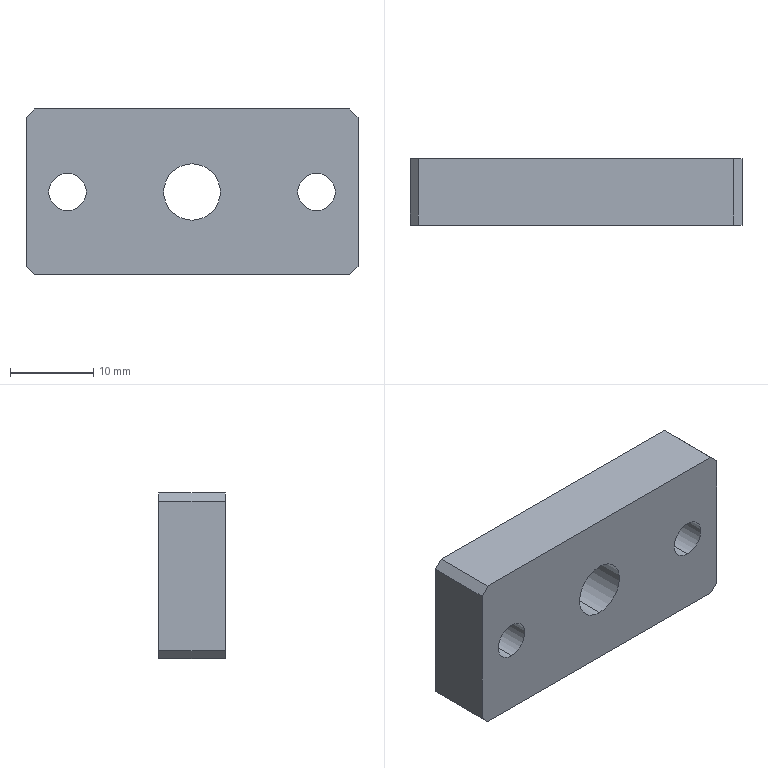Part | NX | features BREP 1 | 1 solid | 22 faces | box 40 x 8 x 20 mm | volume 5530 mm3 | plane 12 | cylinder 10 | commonest cylinder face diameters 4.5 x4 8 x4 6.8 x2
STEP:
#1=CARTESIAN_POINT('',(15.,-4.,-2.25));
#2=VERTEX_POINT('',#1);
#3=CARTESIAN_POINT('',(15.,-4.,2.25));
#4=VERTEX_POINT('',#3);
#5=CARTESIAN_POINT('',(15.,-4.,0.));
#6=DIRECTION('',(0.,1.,0.));
#7=DIRECTION('',(0.,0.,1.));
#8=AXIS2_PLACEMENT_3D('',#5,#6,#7);
#9=CIRCLE('',#8,2.25);
#10=EDGE_CURVE('',#2,#4,#9,.T.);
#11=ORIENTED_EDGE('',*,*,#10,.F.);
#12=CARTESIAN_POINT('',(15.,-0.5,-2.25));
#13=VERTEX_POINT('',#12);
#14=CARTESIAN_POINT('',(15.,4.,-2.25));
#15=DIRECTION('',(0.,1.,0.));
#16=VECTOR('',#15,1000.);
#17=LINE('',#14,#16);
#18=EDGE_CURVE('',#13,#2,#17,.F.);
#19=ORIENTED_EDGE('',*,*,#18,.F.);
#20=CARTESIAN_POINT('',(15.,-0.5,2.25));
#21=VERTEX_POINT('',#20);
#22=CARTESIAN_POINT('',(15.,-0.5,0.));
#23=DIRECTION('',(0.,1.,0.));
#24=DIRECTION('',(0.,0.,1.));
#25=AXIS2_PLACEMENT_3D('',#22,#23,#24);
#26=CIRCLE('',#25,2.25);
#27=EDGE_CURVE('',#13,#21,#26,.T.);
#28=ORIENTED_EDGE('',*,*,#27,.T.);
#29=CARTESIAN_POINT('',(15.,4.,2.25));
#30=DIRECTION('',(0.,1.,0.));
#31=VECTOR('',#30,1000.);
#32=LINE('',#29,#31);
#33=EDGE_CURVE('',#21,#4,#32,.F.);
#34=ORIENTED_EDGE('',*,*,#33,.T.);
#35=EDGE_LOOP('',(#11,#19,#28,#34));
#36=FACE_BOUND('',#35,.T.);
#37=CARTESIAN_POINT('',(15.,4.,0.));
#38=DIRECTION('',(0.,1.,0.));
#39=DIRECTION('',(0.,0.,1.));
#40=AXIS2_PLACEMENT_3D('',#37,#38,#39);
#41=CYLINDRICAL_SURFACE('',#40,2.25);
#42=ADVANCED_FACE('',(#36),#41,.F.);
#43=CARTESIAN_POINT('',(15.,-0.5,-4.));
#44=VERTEX_POINT('',#43);
#45=CARTESIAN_POINT('',(15.,-0.5,4.));
#46=VERTEX_POINT('',#45);
#47=CARTESIAN_POINT('',(15.,-0.5,0.));
#48=DIRECTION('',(0.,1.,0.));
#49=DIRECTION('',(0.,0.,1.));
#50=AXIS2_PLACEMENT_3D('',#47,#48,#49);
#51=CIRCLE('',#50,4.);
#52=EDGE_CURVE('',#44,#46,#51,.T.);
#53=ORIENTED_EDGE('',*,*,#52,.F.);
#54=CARTESIAN_POINT('',(15.,4.,-4.));
#55=VERTEX_POINT('',#54);
#56=CARTESIAN_POINT('',(15.,4.,-4.));
#57=DIRECTION('',(0.,1.,0.));
#58=VECTOR('',#57,1000.);
#59=LINE('',#56,#58);
#60=EDGE_CURVE('',#55,#44,#59,.F.);
#61=ORIENTED_EDGE('',*,*,#60,.F.);
#62=CARTESIAN_POINT('',(15.,4.,4.));
#63=VERTEX_POINT('',#62);
#64=CARTESIAN_POINT('',(15.,4.,0.));
#65=DIRECTION('',(0.,1.,0.));
#66=DIRECTION('',(0.,0.,1.));
#67=AXIS2_PLACEMENT_3D('',#64,#65,#66);
#68=CIRCLE('',#67,4.);
#69=EDGE_CURVE('',#55,#63,#68,.T.);
#70=ORIENTED_EDGE('',*,*,#69,.T.);
#71=CARTESIAN_POINT('',(15.,4.,4.));
#72=DIRECTION('',(0.,1.,0.));
#73=VECTOR('',#72,1000.);
#74=LINE('',#71,#73);
#75=EDGE_CURVE('',#63,#46,#74,.F.);
#76=ORIENTED_EDGE('',*,*,#75,.T.);
#77=EDGE_LOOP('',(#53,#61,#70,#76));
#78=FACE_BOUND('',#77,.T.);
#79=CARTESIAN_POINT('',(15.,4.,0.));
#80=DIRECTION('',(0.,1.,0.));
#81=DIRECTION('',(0.,0.,1.));
#82=AXIS2_PLACEMENT_3D('',#79,#80,#81);
#83=CYLINDRICAL_SURFACE('',#82,4.);
#84=ADVANCED_FACE('',(#78),#83,.F.);
#85=CARTESIAN_POINT('',(-15.,-4.,-2.25));
#86=VERTEX_POINT('',#85);
#87=CARTESIAN_POINT('',(-15.,-4.,2.25));
#88=VERTEX_POINT('',#87);
#89=CARTESIAN_POINT('',(-15.,-4.,0.));
#90=DIRECTION('',(0.,1.,0.));
#91=DIRECTION('',(0.,0.,1.));
#92=AXIS2_PLACEMENT_3D('',#89,#90,#91);
#93=CIRCLE('',#92,2.25);
#94=EDGE_CURVE('',#86,#88,#93,.T.);
#95=ORIENTED_EDGE('',*,*,#94,.F.);
#96=CARTESIAN_POINT('',(-15.,-0.5,-2.25));
#97=VERTEX_POINT('',#96);
#98=CARTESIAN_POINT('',(-15.,4.,-2.25));
#99=DIRECTION('',(0.,1.,0.));
#100=VECTOR('',#99,1000.);
#101=LINE('',#98,#100);
#102=EDGE_CURVE('',#97,#86,#101,.F.);
#103=ORIENTED_EDGE('',*,*,#102,.F.);
#104=CARTESIAN_POINT('',(-15.,-0.5,2.25));
#105=VERTEX_POINT('',#104);
#106=CARTESIAN_POINT('',(-15.,-0.5,0.));
#107=DIRECTION('',(0.,1.,0.));
#108=DIRECTION('',(0.,0.,1.));
#109=AXIS2_PLACEMENT_3D('',#106,#107,#108);
#110=CIRCLE('',#109,2.25);
#111=EDGE_CURVE('',#97,#105,#110,.T.);
#112=ORIENTED_EDGE('',*,*,#111,.T.);
#113=CARTESIAN_POINT('',(-15.,4.,2.25));
#114=DIRECTION('',(0.,1.,0.));
#115=VECTOR('',#114,1000.);
#116=LINE('',#113,#115);
#117=EDGE_CURVE('',#105,#88,#116,.F.);
#118=ORIENTED_EDGE('',*,*,#117,.T.);
#119=EDGE_LOOP('',(#95,#103,#112,#118));
#120=FACE_BOUND('',#119,.T.);
#121=CARTESIAN_POINT('',(-15.,4.,0.));
#122=DIRECTION('',(0.,1.,0.));
#123=DIRECTION('',(0.,0.,1.));
#124=AXIS2_PLACEMENT_3D('',#121,#122,#123);
#125=CYLINDRICAL_SURFACE('',#124,2.25);
#126=ADVANCED_FACE('',(#120),#125,.F.);
#127=CARTESIAN_POINT('',(-15.,-0.5,-4.));
#128=VERTEX_POINT('',#127);
#129=CARTESIAN_POINT('',(-15.,-0.5,4.));
#130=VERTEX_POINT('',#129);
#131=CARTESIAN_POINT('',(-15.,-0.5,0.));
#132=DIRECTION('',(0.,1.,0.));
#133=DIRECTION('',(0.,0.,1.));
#134=AXIS2_PLACEMENT_3D('',#131,#132,#133);
#135=CIRCLE('',#134,4.);
#136=EDGE_CURVE('',#128,#130,#135,.T.);
#137=ORIENTED_EDGE('',*,*,#136,.F.);
#138=CARTESIAN_POINT('',(-15.,4.,-4.));
#139=VERTEX_POINT('',#138);
#140=CARTESIAN_POINT('',(-15.,4.,-4.));
#141=DIRECTION('',(0.,1.,0.));
#142=VECTOR('',#141,1000.);
#143=LINE('',#140,#142);
#144=EDGE_CURVE('',#139,#128,#143,.F.);
#145=ORIENTED_EDGE('',*,*,#144,.F.);
#146=CARTESIAN_POINT('',(-15.,4.,4.));
#147=VERTEX_POINT('',#146);
#148=CARTESIAN_POINT('',(-15.,4.,0.));
#149=DIRECTION('',(0.,1.,0.));
#150=DIRECTION('',(0.,0.,1.));
#151=AXIS2_PLACEMENT_3D('',#148,#149,#150);
#152=CIRCLE('',#151,4.);
#153=EDGE_CURVE('',#139,#147,#152,.T.);
#154=ORIENTED_EDGE('',*,*,#153,.T.);
#155=CARTESIAN_POINT('',(-15.,4.,4.));
#156=DIRECTION('',(0.,1.,0.));
#157=VECTOR('',#156,1000.);
#158=LINE('',#155,#157);
#159=EDGE_CURVE('',#147,#130,#158,.F.);
#160=ORIENTED_EDGE('',*,*,#159,.T.);
#161=EDGE_LOOP('',(#137,#145,#154,#160));
#162=FACE_BOUND('',#161,.T.);
#163=CARTESIAN_POINT('',(-15.,4.,0.));
#164=DIRECTION('',(0.,1.,0.));
#165=DIRECTION('',(0.,0.,1.));
#166=AXIS2_PLACEMENT_3D('',#163,#164,#165);
#167=CYLINDRICAL_SURFACE('',#166,4.);
#168=ADVANCED_FACE('',(#162),#167,.F.);
#169=CARTESIAN_POINT('',(0.,-4.,-3.4));
#170=VERTEX_POINT('',#169);
#171=CARTESIAN_POINT('',(0.,-4.,3.4));
#172=VERTEX_POINT('',#171);
#173=CARTESIAN_POINT('',(0.,-4.,0.));
#174=DIRECTION('',(0.,1.,0.));
#175=DIRECTION('',(0.,0.,1.));
#176=AXIS2_PLACEMENT_3D('',#173,#174,#175);
#177=CIRCLE('',#176,3.4);
#178=EDGE_CURVE('',#170,#172,#177,.T.);
#179=ORIENTED_EDGE('',*,*,#178,.F.);
#180=CARTESIAN_POINT('',(0.,4.,-3.4));
#181=VERTEX_POINT('',#180);
#182=CARTESIAN_POINT('',(0.,4.,-3.4));
#183=DIRECTION('',(0.,1.,0.));
#184=VECTOR('',#183,1000.);
#185=LINE('',#182,#184);
#186=EDGE_CURVE('',#181,#170,#185,.F.);
#187=ORIENTED_EDGE('',*,*,#186,.F.);
#188=CARTESIAN_POINT('',(0.,4.,3.4));
#189=VERTEX_POINT('',#188);
#190=CARTESIAN_POINT('',(0.,4.,0.));
#191=DIRECTION('',(0.,1.,0.));
#192=DIRECTION('',(0.,0.,1.));
#193=AXIS2_PLACEMENT_3D('',#190,#191,#192);
#194=CIRCLE('',#193,3.4);
#195=EDGE_CURVE('',#181,#189,#194,.T.);
#196=ORIENTED_EDGE('',*,*,#195,.T.);
#197=CARTESIAN_POINT('',(0.,4.,3.4));
#198=DIRECTION('',(0.,1.,0.));
#199=VECTOR('',#198,1000.);
#200=LINE('',#197,#199);
#201=EDGE_CURVE('',#189,#172,#200,.F.);
#202=ORIENTED_EDGE('',*,*,#201,.T.);
#203=EDGE_LOOP('',(#179,#187,#196,#202));
#204=FACE_BOUND('',#203,.T.);
#205=CARTESIAN_POINT('',(0.,4.,0.));
#206=DIRECTION('',(0.,1.,0.));
#207=DIRECTION('',(0.,0.,1.));
#208=AXIS2_PLACEMENT_3D('',#205,#206,#207);
#209=CYLINDRICAL_SURFACE('',#208,3.4);
#210=ADVANCED_FACE('',(#204),#209,.F.);
#211=CARTESIAN_POINT('',(19.,-4.,-10.));
#212=VERTEX_POINT('',#211);
#213=CARTESIAN_POINT('',(-19.,-4.,-10.));
#214=VERTEX_POINT('',#213);
#215=CARTESIAN_POINT('',(20.,-4.,-10.));
#216=DIRECTION('',(-1.,0.,0.));
#217=VECTOR('',#216,1000.);
#218=LINE('',#215,#217);
#219=EDGE_CURVE('',#212,#214,#218,.T.);
#220=ORIENTED_EDGE('',*,*,#219,.F.);
#221=CARTESIAN_POINT('',(20.,-4.,-9.));
#222=VERTEX_POINT('',#221);
#223=CARTESIAN_POINT('',(29.5,-4.,0.5));
#224=DIRECTION('',(0.7071,0.,0.7071));
#225=VECTOR('',#224,1000.);
#226=LINE('',#223,#225);
#227=EDGE_CURVE('',#212,#222,#226,.T.);
#228=ORIENTED_EDGE('',*,*,#227,.T.);
#229=CARTESIAN_POINT('',(20.,-4.,9.));
#230=VERTEX_POINT('',#229);
#231=CARTESIAN_POINT('',(20.,-4.,-10.));
#232=DIRECTION('',(0.,0.,-1.));
#233=VECTOR('',#232,1000.);
#234=LINE('',#231,#233);
#235=EDGE_CURVE('',#230,#222,#234,.T.);
#236=ORIENTED_EDGE('',*,*,#235,.F.);
#237=CARTESIAN_POINT('',(19.,-4.,10.));
#238=VERTEX_POINT('',#237);
#239=CARTESIAN_POINT('',(19.5,-4.,9.5));
#240=DIRECTION('',(-0.7071,0.,0.7071));
#241=VECTOR('',#240,1000.);
#242=LINE('',#239,#241);
#243=EDGE_CURVE('',#230,#238,#242,.T.);
#244=ORIENTED_EDGE('',*,*,#243,.T.);
#245=CARTESIAN_POINT('',(-19.,-4.,10.));
#246=VERTEX_POINT('',#245);
#247=CARTESIAN_POINT('',(20.,-4.,10.));
#248=DIRECTION('',(1.,0.,0.));
#249=VECTOR('',#248,1000.);
#250=LINE('',#247,#249);
#251=EDGE_CURVE('',#246,#238,#250,.T.);
#252=ORIENTED_EDGE('',*,*,#251,.F.);
#253=CARTESIAN_POINT('',(-20.,-4.,9.));
#254=VERTEX_POINT('',#253);
#255=CARTESIAN_POINT('',(0.5,-4.,29.5));
#256=DIRECTION('',(-0.7071,0.,-0.7071));
#257=VECTOR('',#256,1000.);
#258=LINE('',#255,#257);
#259=EDGE_CURVE('',#246,#254,#258,.T.);
#260=ORIENTED_EDGE('',*,*,#259,.T.);
#261=CARTESIAN_POINT('',(-20.,-4.,-9.));
#262=VERTEX_POINT('',#261);
#263=CARTESIAN_POINT('',(-20.,-4.,-10.));
#264=DIRECTION('',(0.,0.,1.));
#265=VECTOR('',#264,1000.);
#266=LINE('',#263,#265);
#267=EDGE_CURVE('',#262,#254,#266,.T.);
#268=ORIENTED_EDGE('',*,*,#267,.F.);
#269=CARTESIAN_POINT('',(-9.5,-4.,-19.5));
#270=DIRECTION('',(0.7071,0.,-0.7071));
#271=VECTOR('',#270,1000.);
#272=LINE('',#269,#271);
#273=EDGE_CURVE('',#262,#214,#272,.T.);
#274=ORIENTED_EDGE('',*,*,#273,.T.);
#275=EDGE_LOOP('',(#220,#228,#236,#244,#252,#260,#268,#274));
#276=FACE_BOUND('',#275,.T.);
#277=CARTESIAN_POINT('',(-15.,-4.,0.));
#278=DIRECTION('',(0.,1.,0.));
#279=DIRECTION('',(0.,0.,1.));
#280=AXIS2_PLACEMENT_3D('',#277,#278,#279);
#281=CIRCLE('',#280,2.25);
#282=EDGE_CURVE('',#88,#86,#281,.T.);
#283=ORIENTED_EDGE('',*,*,#282,.T.);
#284=ORIENTED_EDGE('',*,*,#94,.T.);
#285=EDGE_LOOP('',(#283,#284));
#286=FACE_BOUND('',#285,.T.);
#287=CARTESIAN_POINT('',(0.,-4.,0.));
#288=DIRECTION('',(0.,1.,0.));
#289=DIRECTION('',(0.,0.,1.));
#290=AXIS2_PLACEMENT_3D('',#287,#288,#289);
#291=CIRCLE('',#290,3.4);
#292=EDGE_CURVE('',#172,#170,#291,.T.);
#293=ORIENTED_EDGE('',*,*,#292,.T.);
#294=ORIENTED_EDGE('',*,*,#178,.T.);
#295=EDGE_LOOP('',(#293,#294));
#296=FACE_BOUND('',#295,.T.);
#297=CARTESIAN_POINT('',(15.,-4.,0.));
#298=DIRECTION('',(0.,1.,0.));
#299=DIRECTION('',(0.,0.,1.));
#300=AXIS2_PLACEMENT_3D('',#297,#298,#299);
#301=CIRCLE('',#300,2.25);
#302=EDGE_CURVE('',#4,#2,#301,.T.);
#303=ORIENTED_EDGE('',*,*,#302,.T.);
#304=ORIENTED_EDGE('',*,*,#10,.T.);
#305=EDGE_LOOP('',(#303,#304));
#306=FACE_BOUND('',#305,.T.);
#307=CARTESIAN_POINT('',(20.,-4.,10.));
#308=DIRECTION('',(0.,-1.,0.));
#309=DIRECTION('',(0.,0.,-1.));
#310=AXIS2_PLACEMENT_3D('',#307,#308,#309);
#311=PLANE('',#310);
#312=ADVANCED_FACE('',(#276,#286,#296,#306),#311,.T.);
#313=ORIENTED_EDGE('',*,*,#235,.T.);
#314=CARTESIAN_POINT('',(20.,4.,-9.));
#315=VERTEX_POINT('',#314);
#316=CARTESIAN_POINT('',(20.,4.,-9.));
#317=DIRECTION('',(0.,1.,0.));
#318=VECTOR('',#317,1000.);
#319=LINE('',#316,#318);
#320=EDGE_CURVE('',#222,#315,#319,.T.);
#321=ORIENTED_EDGE('',*,*,#320,.T.);
#322=CARTESIAN_POINT('',(20.,4.,9.));
#323=VERTEX_POINT('',#322);
#324=CARTESIAN_POINT('',(20.,4.,-10.));
#325=DIRECTION('',(0.,0.,-1.));
#326=VECTOR('',#325,1000.);
#327=LINE('',#324,#326);
#328=EDGE_CURVE('',#323,#315,#327,.T.);
#329=ORIENTED_EDGE('',*,*,#328,.F.);
#330=CARTESIAN_POINT('',(20.,4.,9.));
#331=DIRECTION('',(0.,-1.,0.));
#332=VECTOR('',#331,1000.);
#333=LINE('',#330,#332);
#334=EDGE_CURVE('',#323,#230,#333,.T.);
#335=ORIENTED_EDGE('',*,*,#334,.T.);
#336=EDGE_LOOP('',(#313,#321,#329,#335));
#337=FACE_BOUND('',#336,.T.);
#338=CARTESIAN_POINT('',(20.,4.,-10.));
#339=DIRECTION('',(-1.,0.,0.));
#340=DIRECTION('',(0.,0.,1.));
#341=AXIS2_PLACEMENT_3D('',#338,#339,#340);
#342=PLANE('',#341);
#343=ADVANCED_FACE('',(#337),#342,.F.);
#344=CARTESIAN_POINT('',(19.,4.,-10.));
#345=VERTEX_POINT('',#344);
#346=CARTESIAN_POINT('',(-19.,4.,-10.));
#347=VERTEX_POINT('',#346);
#348=CARTESIAN_POINT('',(20.,4.,-10.));
#349=DIRECTION('',(-1.,0.,0.));
#350=VECTOR('',#349,1000.);
#351=LINE('',#348,#350);
#352=EDGE_CURVE('',#345,#347,#351,.T.);
#353=ORIENTED_EDGE('',*,*,#352,.F.);
#354=CARTESIAN_POINT('',(19.,4.,-10.));
#355=DIRECTION('',(0.,-1.,0.));
#356=VECTOR('',#355,1000.);
#357=LINE('',#354,#356);
#358=EDGE_CURVE('',#345,#212,#357,.T.);
#359=ORIENTED_EDGE('',*,*,#358,.T.);
#360=ORIENTED_EDGE('',*,*,#219,.T.);
#361=CARTESIAN_POINT('',(-19.,4.,-10.));
#362=DIRECTION('',(0.,1.,0.));
#363=VECTOR('',#362,1000.);
#364=LINE('',#361,#363);
#365=EDGE_CURVE('',#214,#347,#364,.T.);
#366=ORIENTED_EDGE('',*,*,#365,.T.);
#367=EDGE_LOOP('',(#353,#359,#360,#366));
#368=FACE_BOUND('',#367,.T.);
#369=CARTESIAN_POINT('',(20.,4.,-10.));
#370=DIRECTION('',(0.,0.,1.));
#371=DIRECTION('',(1.,0.,0.));
#372=AXIS2_PLACEMENT_3D('',#369,#370,#371);
#373=PLANE('',#372);
#374=ADVANCED_FACE('',(#368),#373,.F.);
#375=CARTESIAN_POINT('',(-20.,4.,-9.));
#376=VERTEX_POINT('',#375);
#377=CARTESIAN_POINT('',(-20.,4.,9.));
#378=VERTEX_POINT('',#377);
#379=CARTESIAN_POINT('',(-20.,4.,-10.));
#380=DIRECTION('',(0.,0.,1.));
#381=VECTOR('',#380,1000.);
#382=LINE('',#379,#381);
#383=EDGE_CURVE('',#376,#378,#382,.T.);
#384=ORIENTED_EDGE('',*,*,#383,.F.);
#385=CARTESIAN_POINT('',(-20.,4.,-9.));
#386=DIRECTION('',(0.,-1.,0.));
#387=VECTOR('',#386,1000.);
#388=LINE('',#385,#387);
#389=EDGE_CURVE('',#376,#262,#388,.T.);
#390=ORIENTED_EDGE('',*,*,#389,.T.);
#391=ORIENTED_EDGE('',*,*,#267,.T.);
#392=CARTESIAN_POINT('',(-20.,4.,9.));
#393=DIRECTION('',(0.,1.,0.));
#394=VECTOR('',#393,1000.);
#395=LINE('',#392,#394);
#396=EDGE_CURVE('',#254,#378,#395,.T.);
#397=ORIENTED_EDGE('',*,*,#396,.T.);
#398=EDGE_LOOP('',(#384,#390,#391,#397));
#399=FACE_BOUND('',#398,.T.);
#400=CARTESIAN_POINT('',(-20.,4.,-10.));
#401=DIRECTION('',(1.,0.,0.));
#402=DIRECTION('',(0.,0.,1.));
#403=AXIS2_PLACEMENT_3D('',#400,#401,#402);
#404=PLANE('',#403);
#405=ADVANCED_FACE('',(#399),#404,.F.);
#406=ORIENTED_EDGE('',*,*,#251,.T.);
#407=CARTESIAN_POINT('',(19.,4.,10.));
#408=VERTEX_POINT('',#407);
#409=CARTESIAN_POINT('',(19.,4.,10.));
#410=DIRECTION('',(0.,1.,0.));
#411=VECTOR('',#410,1000.);
#412=LINE('',#409,#411);
#413=EDGE_CURVE('',#238,#408,#412,.T.);
#414=ORIENTED_EDGE('',*,*,#413,.T.);
#415=CARTESIAN_POINT('',(-19.,4.,10.));
#416=VERTEX_POINT('',#415);
#417=CARTESIAN_POINT('',(20.,4.,10.));
#418=DIRECTION('',(1.,0.,0.));
#419=VECTOR('',#418,1000.);
#420=LINE('',#417,#419);
#421=EDGE_CURVE('',#416,#408,#420,.T.);
#422=ORIENTED_EDGE('',*,*,#421,.F.);
#423=CARTESIAN_POINT('',(-19.,4.,10.));
#424=DIRECTION('',(0.,-1.,0.));
#425=VECTOR('',#424,1000.);
#426=LINE('',#423,#425);
#427=EDGE_CURVE('',#416,#246,#426,.T.);
#428=ORIENTED_EDGE('',*,*,#427,.T.);
#429=EDGE_LOOP('',(#406,#414,#422,#428));
#430=FACE_BOUND('',#429,.T.);
#431=CARTESIAN_POINT('',(20.,4.,10.));
#432=DIRECTION('',(0.,0.,-1.));
#433=DIRECTION('',(-1.,0.,0.));
#434=AXIS2_PLACEMENT_3D('',#431,#432,#433);
#435=PLANE('',#434);
#436=ADVANCED_FACE('',(#430),#435,.F.);
#437=ORIENTED_EDGE('',*,*,#328,.T.);
#438=CARTESIAN_POINT('',(19.,4.,-10.));
#439=DIRECTION('',(-0.7071,0.,-0.7071));
#440=VECTOR('',#439,1000.);
#441=LINE('',#438,#440);
#442=EDGE_CURVE('',#315,#345,#441,.T.);
#443=ORIENTED_EDGE('',*,*,#442,.T.);
#444=ORIENTED_EDGE('',*,*,#352,.T.);
#445=CARTESIAN_POINT('',(-20.,4.,-9.));
#446=DIRECTION('',(-0.7071,0.,0.7071));
#447=VECTOR('',#446,1000.);
#448=LINE('',#445,#447);
#449=EDGE_CURVE('',#347,#376,#448,.T.);
#450=ORIENTED_EDGE('',*,*,#449,.T.);
#451=ORIENTED_EDGE('',*,*,#383,.T.);
#452=CARTESIAN_POINT('',(-19.,4.,10.));
#453=DIRECTION('',(0.7071,0.,0.7071));
#454=VECTOR('',#453,1000.);
#455=LINE('',#452,#454);
#456=EDGE_CURVE('',#378,#416,#455,.T.);
#457=ORIENTED_EDGE('',*,*,#456,.T.);
#458=ORIENTED_EDGE('',*,*,#421,.T.);
#459=CARTESIAN_POINT('',(20.,4.,9.));
#460=DIRECTION('',(0.7071,0.,-0.7071));
#461=VECTOR('',#460,1000.);
#462=LINE('',#459,#461);
#463=EDGE_CURVE('',#408,#323,#462,.T.);
#464=ORIENTED_EDGE('',*,*,#463,.T.);
#465=EDGE_LOOP('',(#437,#443,#444,#450,#451,#457,#458,#464));
#466=FACE_BOUND('',#465,.T.);
#467=CARTESIAN_POINT('',(15.,4.,0.));
#468=DIRECTION('',(0.,1.,0.));
#469=DIRECTION('',(0.,0.,1.));
#470=AXIS2_PLACEMENT_3D('',#467,#468,#469);
#471=CIRCLE('',#470,4.);
#472=EDGE_CURVE('',#63,#55,#471,.T.);
#473=ORIENTED_EDGE('',*,*,#472,.F.);
#474=ORIENTED_EDGE('',*,*,#69,.F.);
#475=EDGE_LOOP('',(#473,#474));
#476=FACE_BOUND('',#475,.T.);
#477=CARTESIAN_POINT('',(-15.,4.,0.));
#478=DIRECTION('',(0.,1.,0.));
#479=DIRECTION('',(0.,0.,1.));
#480=AXIS2_PLACEMENT_3D('',#477,#478,#479);
#481=CIRCLE('',#480,4.);
#482=EDGE_CURVE('',#147,#139,#481,.T.);
#483=ORIENTED_EDGE('',*,*,#482,.F.);
#484=ORIENTED_EDGE('',*,*,#153,.F.);
#485=EDGE_LOOP('',(#483,#484));
#486=FACE_BOUND('',#485,.T.);
#487=CARTESIAN_POINT('',(0.,4.,0.));
#488=DIRECTION('',(0.,1.,0.));
#489=DIRECTION('',(0.,0.,1.));
#490=AXIS2_PLACEMENT_3D('',#487,#488,#489);
#491=CIRCLE('',#490,3.4);
#492=EDGE_CURVE('',#189,#181,#491,.T.);
#493=ORIENTED_EDGE('',*,*,#492,.F.);
#494=ORIENTED_EDGE('',*,*,#195,.F.);
#495=EDGE_LOOP('',(#493,#494));
#496=FACE_BOUND('',#495,.T.);
#497=CARTESIAN_POINT('',(20.,4.,10.));
#498=DIRECTION('',(0.,-1.,0.));
#499=DIRECTION('',(0.,0.,-1.));
#500=AXIS2_PLACEMENT_3D('',#497,#498,#499);
#501=PLANE('',#500);
#502=ADVANCED_FACE('',(#466,#476,#486,#496),#501,.F.);
#503=ORIENTED_EDGE('',*,*,#442,.F.);
#504=ORIENTED_EDGE('',*,*,#320,.F.);
#505=ORIENTED_EDGE('',*,*,#227,.F.);
#506=ORIENTED_EDGE('',*,*,#358,.F.);
#507=EDGE_LOOP('',(#503,#504,#505,#506));
#508=FACE_BOUND('',#507,.T.);
#509=CARTESIAN_POINT('',(19.,4.,-10.));
#510=DIRECTION('',(-0.7071,0.,0.7071));
#511=DIRECTION('',(0.,1.,0.));
#512=AXIS2_PLACEMENT_3D('',#509,#510,#511);
#513=PLANE('',#512);
#514=ADVANCED_FACE('',(#508),#513,.F.);
#515=ORIENTED_EDGE('',*,*,#463,.F.);
#516=ORIENTED_EDGE('',*,*,#413,.F.);
#517=ORIENTED_EDGE('',*,*,#243,.F.);
#518=ORIENTED_EDGE('',*,*,#334,.F.);
#519=EDGE_LOOP('',(#515,#516,#517,#518));
#520=FACE_BOUND('',#519,.T.);
#521=CARTESIAN_POINT('',(20.,4.,9.));
#522=DIRECTION('',(-0.7071,0.,-0.7071));
#523=DIRECTION('',(-0.7071,0.,0.7071));
#524=AXIS2_PLACEMENT_3D('',#521,#522,#523);
#525=PLANE('',#524);
#526=ADVANCED_FACE('',(#520),#525,.F.);
#527=ORIENTED_EDGE('',*,*,#449,.F.);
#528=ORIENTED_EDGE('',*,*,#365,.F.);
#529=ORIENTED_EDGE('',*,*,#273,.F.);
#530=ORIENTED_EDGE('',*,*,#389,.F.);
#531=EDGE_LOOP('',(#527,#528,#529,#530));
#532=FACE_BOUND('',#531,.T.);
#533=CARTESIAN_POINT('',(-20.,4.,-9.));
#534=DIRECTION('',(0.7071,0.,0.7071));
#535=DIRECTION('',(0.,-1.,0.));
#536=AXIS2_PLACEMENT_3D('',#533,#534,#535);
#537=PLANE('',#536);
#538=ADVANCED_FACE('',(#532),#537,.F.);
#539=ORIENTED_EDGE('',*,*,#456,.F.);
#540=ORIENTED_EDGE('',*,*,#396,.F.);
#541=ORIENTED_EDGE('',*,*,#259,.F.);
#542=ORIENTED_EDGE('',*,*,#427,.F.);
#543=EDGE_LOOP('',(#539,#540,#541,#542));
#544=FACE_BOUND('',#543,.T.);
#545=CARTESIAN_POINT('',(-19.,4.,10.));
#546=DIRECTION('',(0.7071,0.,-0.7071));
#547=DIRECTION('',(0.,-1.,0.));
#548=AXIS2_PLACEMENT_3D('',#545,#546,#547);
#549=PLANE('',#548);
#550=ADVANCED_FACE('',(#544),#549,.F.);
#551=ORIENTED_EDGE('',*,*,#186,.T.);
#552=ORIENTED_EDGE('',*,*,#292,.F.);
#553=ORIENTED_EDGE('',*,*,#201,.F.);
#554=ORIENTED_EDGE('',*,*,#492,.T.);
#555=EDGE_LOOP('',(#551,#552,#553,#554));
#556=FACE_BOUND('',#555,.T.);
#557=CARTESIAN_POINT('',(0.,4.,0.));
#558=DIRECTION('',(0.,1.,0.));
#559=DIRECTION('',(0.,0.,1.));
#560=AXIS2_PLACEMENT_3D('',#557,#558,#559);
#561=CYLINDRICAL_SURFACE('',#560,3.4);
#562=ADVANCED_FACE('',(#556),#561,.F.);
#563=ORIENTED_EDGE('',*,*,#144,.T.);
#564=CARTESIAN_POINT('',(-15.,-0.5,0.));
#565=DIRECTION('',(0.,1.,0.));
#566=DIRECTION('',(0.,0.,1.));
#567=AXIS2_PLACEMENT_3D('',#564,#565,#566);
#568=CIRCLE('',#567,4.);
#569=EDGE_CURVE('',#130,#128,#568,.T.);
#570=ORIENTED_EDGE('',*,*,#569,.F.);
#571=ORIENTED_EDGE('',*,*,#159,.F.);
#572=ORIENTED_EDGE('',*,*,#482,.T.);
#573=EDGE_LOOP('',(#563,#570,#571,#572));
#574=FACE_BOUND('',#573,.T.);
#575=CARTESIAN_POINT('',(-15.,4.,0.));
#576=DIRECTION('',(0.,1.,0.));
#577=DIRECTION('',(0.,0.,1.));
#578=AXIS2_PLACEMENT_3D('',#575,#576,#577);
#579=CYLINDRICAL_SURFACE('',#578,4.);
#580=ADVANCED_FACE('',(#574),#579,.F.);
#581=ORIENTED_EDGE('',*,*,#569,.T.);
#582=ORIENTED_EDGE('',*,*,#136,.T.);
#583=EDGE_LOOP('',(#581,#582));
#584=FACE_BOUND('',#583,.T.);
#585=CARTESIAN_POINT('',(-15.,-0.5,0.));
#586=DIRECTION('',(0.,1.,0.));
#587=DIRECTION('',(0.,0.,1.));
#588=AXIS2_PLACEMENT_3D('',#585,#586,#587);
#589=CIRCLE('',#588,2.25);
#590=EDGE_CURVE('',#105,#97,#589,.T.);
#591=ORIENTED_EDGE('',*,*,#590,.F.);
#592=ORIENTED_EDGE('',*,*,#111,.F.);
#593=EDGE_LOOP('',(#591,#592));
#594=FACE_BOUND('',#593,.T.);
#595=CARTESIAN_POINT('',(-12.75,-0.5,0.));
#596=DIRECTION('',(0.,-1.,0.));
#597=DIRECTION('',(0.,0.,-1.));
#598=AXIS2_PLACEMENT_3D('',#595,#596,#597);
#599=PLANE('',#598);
#600=ADVANCED_FACE('',(#584,#594),#599,.F.);
#601=ORIENTED_EDGE('',*,*,#102,.T.);
#602=ORIENTED_EDGE('',*,*,#282,.F.);
#603=ORIENTED_EDGE('',*,*,#117,.F.);
#604=ORIENTED_EDGE('',*,*,#590,.T.);
#605=EDGE_LOOP('',(#601,#602,#603,#604));
#606=FACE_BOUND('',#605,.T.);
#607=CARTESIAN_POINT('',(-15.,4.,0.));
#608=DIRECTION('',(0.,1.,0.));
#609=DIRECTION('',(0.,0.,1.));
#610=AXIS2_PLACEMENT_3D('',#607,#608,#609);
#611=CYLINDRICAL_SURFACE('',#610,2.25);
#612=ADVANCED_FACE('',(#606),#611,.F.);
#613=ORIENTED_EDGE('',*,*,#60,.T.);
#614=CARTESIAN_POINT('',(15.,-0.5,0.));
#615=DIRECTION('',(0.,1.,0.));
#616=DIRECTION('',(0.,0.,1.));
#617=AXIS2_PLACEMENT_3D('',#614,#615,#616);
#618=CIRCLE('',#617,4.);
#619=EDGE_CURVE('',#46,#44,#618,.T.);
#620=ORIENTED_EDGE('',*,*,#619,.F.);
#621=ORIENTED_EDGE('',*,*,#75,.F.);
#622=ORIENTED_EDGE('',*,*,#472,.T.);
#623=EDGE_LOOP('',(#613,#620,#621,#622));
#624=FACE_BOUND('',#623,.T.);
#625=CARTESIAN_POINT('',(15.,4.,0.));
#626=DIRECTION('',(0.,1.,0.));
#627=DIRECTION('',(0.,0.,1.));
#628=AXIS2_PLACEMENT_3D('',#625,#626,#627);
#629=CYLINDRICAL_SURFACE('',#628,4.);
#630=ADVANCED_FACE('',(#624),#629,.F.);
#631=ORIENTED_EDGE('',*,*,#619,.T.);
#632=ORIENTED_EDGE('',*,*,#52,.T.);
#633=EDGE_LOOP('',(#631,#632));
#634=FACE_BOUND('',#633,.T.);
#635=CARTESIAN_POINT('',(15.,-0.5,0.));
#636=DIRECTION('',(0.,1.,0.));
#637=DIRECTION('',(0.,0.,1.));
#638=AXIS2_PLACEMENT_3D('',#635,#636,#637);
#639=CIRCLE('',#638,2.25);
#640=EDGE_CURVE('',#21,#13,#639,.T.);
#641=ORIENTED_EDGE('',*,*,#640,.F.);
#642=ORIENTED_EDGE('',*,*,#27,.F.);
#643=EDGE_LOOP('',(#641,#642));
#644=FACE_BOUND('',#643,.T.);
#645=CARTESIAN_POINT('',(17.25,-0.5,0.));
#646=DIRECTION('',(0.,-1.,0.));
#647=DIRECTION('',(0.,0.,-1.));
#648=AXIS2_PLACEMENT_3D('',#645,#646,#647);
#649=PLANE('',#648);
#650=ADVANCED_FACE('',(#634,#644),#649,.F.);
#651=ORIENTED_EDGE('',*,*,#18,.T.);
#652=ORIENTED_EDGE('',*,*,#302,.F.);
#653=ORIENTED_EDGE('',*,*,#33,.F.);
#654=ORIENTED_EDGE('',*,*,#640,.T.);
#655=EDGE_LOOP('',(#651,#652,#653,#654));
#656=FACE_BOUND('',#655,.T.);
#657=CARTESIAN_POINT('',(15.,4.,0.));
#658=DIRECTION('',(0.,1.,0.));
#659=DIRECTION('',(0.,0.,1.));
#660=AXIS2_PLACEMENT_3D('',#657,#658,#659);
#661=CYLINDRICAL_SURFACE('',#660,2.25);
#662=ADVANCED_FACE('',(#656),#661,.F.);
#663=CLOSED_SHELL('',(#42,#84,#126,#168,#210,#312,#343,#374,#405,#436,#502,#514,#526,#538,#550,#562,#580,#600,#612,#630,#650,#662));
#664=MANIFOLD_SOLID_BREP('',#663);
#665=(LENGTH_UNIT()NAMED_UNIT(*)SI_UNIT(.MILLI.,.METRE.));
#666=UNCERTAINTY_MEASURE_WITH_UNIT(LENGTH_MEASURE(0.00001),#665,'','');
#667=(NAMED_UNIT(*)PLANE_ANGLE_UNIT()SI_UNIT($,.RADIAN.));
#668=(NAMED_UNIT(*)SI_UNIT($,.STERADIAN.)SOLID_ANGLE_UNIT());
#669=(GEOMETRIC_REPRESENTATION_CONTEXT(3)GLOBAL_UNCERTAINTY_ASSIGNED_CONTEXT((#666))GLOBAL_UNIT_ASSIGNED_CONTEXT((#665,#667,#668))REPRESENTATION_CONTEXT('',''));
#670=ADVANCED_BREP_SHAPE_REPRESENTATION('',(#664),#669);